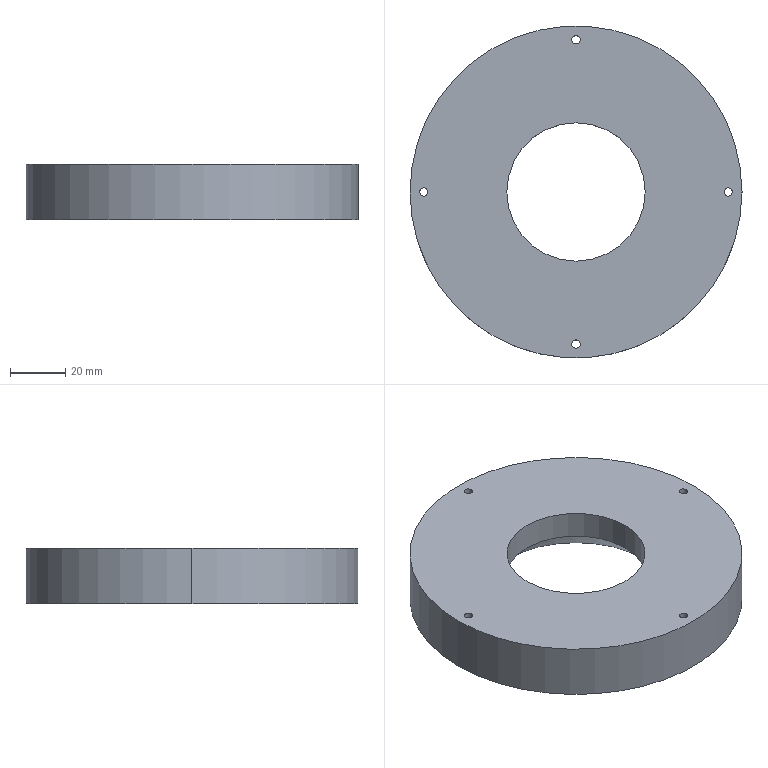Part | SolidWorks | features Chamfer 1, Extrusion 1, ICE 1 | 1 solid | 16 faces | box 120 x 120 x 20 mm | volume 177458 mm3 | cylinder 12 | cone 2 | plane 2 | commonest cylinder face diameters 3 x8 50 x2 120 x2
STEP:
#1=CARTESIAN_POINT('',(-1.5,55.,0.));
#2=VERTEX_POINT('',#1);
#3=CARTESIAN_POINT('',(1.5,55.,0.));
#4=VERTEX_POINT('',#3);
#5=CARTESIAN_POINT('',(0.,55.,0.));
#6=DIRECTION('',(0.,0.,1.));
#7=DIRECTION('',(1.,0.,0.));
#8=AXIS2_PLACEMENT_3D('',#5,#6,#7);
#9=CIRCLE('',#8,1.5);
#10=EDGE_CURVE('',#2,#4,#9,.T.);
#11=ORIENTED_EDGE('',*,*,#10,.F.);
#12=CARTESIAN_POINT('',(-1.5,55.,20.));
#13=VERTEX_POINT('',#12);
#14=CARTESIAN_POINT('',(-1.5,55.,-7.));
#15=DIRECTION('',(0.,0.,1.));
#16=VECTOR('',#15,1000.);
#17=LINE('',#14,#16);
#18=EDGE_CURVE('',#2,#13,#17,.T.);
#19=ORIENTED_EDGE('',*,*,#18,.T.);
#20=CARTESIAN_POINT('',(1.5,55.,20.));
#21=VERTEX_POINT('',#20);
#22=CARTESIAN_POINT('',(0.,55.,20.));
#23=DIRECTION('',(0.,0.,1.));
#24=DIRECTION('',(1.,0.,0.));
#25=AXIS2_PLACEMENT_3D('',#22,#23,#24);
#26=CIRCLE('',#25,1.5);
#27=EDGE_CURVE('',#13,#21,#26,.T.);
#28=ORIENTED_EDGE('',*,*,#27,.T.);
#29=CARTESIAN_POINT('',(1.5,55.,-7.));
#30=DIRECTION('',(0.,0.,1.));
#31=VECTOR('',#30,1000.);
#32=LINE('',#29,#31);
#33=EDGE_CURVE('',#4,#21,#32,.T.);
#34=ORIENTED_EDGE('',*,*,#33,.F.);
#35=EDGE_LOOP('',(#11,#19,#28,#34));
#36=FACE_OUTER_BOUND('',#35,.T.);
#37=CARTESIAN_POINT('',(0.,55.,-7.));
#38=DIRECTION('',(0.,0.,1.));
#39=DIRECTION('',(1.,0.,0.));
#40=AXIS2_PLACEMENT_3D('',#37,#38,#39);
#41=CYLINDRICAL_SURFACE('',#40,1.5);
#42=ADVANCED_FACE('',(#36),#41,.F.);
#43=CARTESIAN_POINT('',(53.5,0.,0.));
#44=VERTEX_POINT('',#43);
#45=CARTESIAN_POINT('',(56.5,0.,0.));
#46=VERTEX_POINT('',#45);
#47=CARTESIAN_POINT('',(55.,0.,0.));
#48=DIRECTION('',(0.,0.,1.));
#49=DIRECTION('',(1.,0.,0.));
#50=AXIS2_PLACEMENT_3D('',#47,#48,#49);
#51=CIRCLE('',#50,1.5);
#52=EDGE_CURVE('',#44,#46,#51,.T.);
#53=ORIENTED_EDGE('',*,*,#52,.F.);
#54=CARTESIAN_POINT('',(53.5,0.,20.));
#55=VERTEX_POINT('',#54);
#56=CARTESIAN_POINT('',(53.5,0.,-7.));
#57=DIRECTION('',(0.,0.,1.));
#58=VECTOR('',#57,1000.);
#59=LINE('',#56,#58);
#60=EDGE_CURVE('',#44,#55,#59,.T.);
#61=ORIENTED_EDGE('',*,*,#60,.T.);
#62=CARTESIAN_POINT('',(56.5,0.,20.));
#63=VERTEX_POINT('',#62);
#64=CARTESIAN_POINT('',(55.,0.,20.));
#65=DIRECTION('',(0.,0.,1.));
#66=DIRECTION('',(1.,0.,0.));
#67=AXIS2_PLACEMENT_3D('',#64,#65,#66);
#68=CIRCLE('',#67,1.5);
#69=EDGE_CURVE('',#55,#63,#68,.T.);
#70=ORIENTED_EDGE('',*,*,#69,.T.);
#71=CARTESIAN_POINT('',(56.5,0.,-7.));
#72=DIRECTION('',(0.,0.,1.));
#73=VECTOR('',#72,1000.);
#74=LINE('',#71,#73);
#75=EDGE_CURVE('',#46,#63,#74,.T.);
#76=ORIENTED_EDGE('',*,*,#75,.F.);
#77=EDGE_LOOP('',(#53,#61,#70,#76));
#78=FACE_OUTER_BOUND('',#77,.T.);
#79=CARTESIAN_POINT('',(55.,0.,-7.));
#80=DIRECTION('',(0.,0.,1.));
#81=DIRECTION('',(1.,0.,0.));
#82=AXIS2_PLACEMENT_3D('',#79,#80,#81);
#83=CYLINDRICAL_SURFACE('',#82,1.5);
#84=ADVANCED_FACE('',(#78),#83,.F.);
#85=CARTESIAN_POINT('',(-1.5,-55.,0.));
#86=VERTEX_POINT('',#85);
#87=CARTESIAN_POINT('',(1.5,-55.,0.));
#88=VERTEX_POINT('',#87);
#89=CARTESIAN_POINT('',(0.,-55.,0.));
#90=DIRECTION('',(0.,0.,1.));
#91=DIRECTION('',(1.,0.,0.));
#92=AXIS2_PLACEMENT_3D('',#89,#90,#91);
#93=CIRCLE('',#92,1.5);
#94=EDGE_CURVE('',#86,#88,#93,.T.);
#95=ORIENTED_EDGE('',*,*,#94,.F.);
#96=CARTESIAN_POINT('',(-1.5,-55.,20.));
#97=VERTEX_POINT('',#96);
#98=CARTESIAN_POINT('',(-1.5,-55.,-7.));
#99=DIRECTION('',(0.,0.,1.));
#100=VECTOR('',#99,1000.);
#101=LINE('',#98,#100);
#102=EDGE_CURVE('',#86,#97,#101,.T.);
#103=ORIENTED_EDGE('',*,*,#102,.T.);
#104=CARTESIAN_POINT('',(1.5,-55.,20.));
#105=VERTEX_POINT('',#104);
#106=CARTESIAN_POINT('',(0.,-55.,20.));
#107=DIRECTION('',(0.,0.,1.));
#108=DIRECTION('',(1.,0.,0.));
#109=AXIS2_PLACEMENT_3D('',#106,#107,#108);
#110=CIRCLE('',#109,1.5);
#111=EDGE_CURVE('',#97,#105,#110,.T.);
#112=ORIENTED_EDGE('',*,*,#111,.T.);
#113=CARTESIAN_POINT('',(1.5,-55.,-7.));
#114=DIRECTION('',(0.,0.,1.));
#115=VECTOR('',#114,1000.);
#116=LINE('',#113,#115);
#117=EDGE_CURVE('',#88,#105,#116,.T.);
#118=ORIENTED_EDGE('',*,*,#117,.F.);
#119=EDGE_LOOP('',(#95,#103,#112,#118));
#120=FACE_OUTER_BOUND('',#119,.T.);
#121=CARTESIAN_POINT('',(0.,-55.,-7.));
#122=DIRECTION('',(0.,0.,1.));
#123=DIRECTION('',(1.,0.,0.));
#124=AXIS2_PLACEMENT_3D('',#121,#122,#123);
#125=CYLINDRICAL_SURFACE('',#124,1.5);
#126=ADVANCED_FACE('',(#120),#125,.F.);
#127=CARTESIAN_POINT('',(-56.5,0.,0.));
#128=VERTEX_POINT('',#127);
#129=CARTESIAN_POINT('',(-53.5,0.,0.));
#130=VERTEX_POINT('',#129);
#131=CARTESIAN_POINT('',(-55.,0.,0.));
#132=DIRECTION('',(0.,0.,1.));
#133=DIRECTION('',(1.,0.,0.));
#134=AXIS2_PLACEMENT_3D('',#131,#132,#133);
#135=CIRCLE('',#134,1.5);
#136=EDGE_CURVE('',#128,#130,#135,.T.);
#137=ORIENTED_EDGE('',*,*,#136,.F.);
#138=CARTESIAN_POINT('',(-56.5,0.,20.));
#139=VERTEX_POINT('',#138);
#140=CARTESIAN_POINT('',(-56.5,0.,-7.));
#141=DIRECTION('',(0.,0.,1.));
#142=VECTOR('',#141,1000.);
#143=LINE('',#140,#142);
#144=EDGE_CURVE('',#128,#139,#143,.T.);
#145=ORIENTED_EDGE('',*,*,#144,.T.);
#146=CARTESIAN_POINT('',(-53.5,0.,20.));
#147=VERTEX_POINT('',#146);
#148=CARTESIAN_POINT('',(-55.,0.,20.));
#149=DIRECTION('',(0.,0.,1.));
#150=DIRECTION('',(1.,0.,0.));
#151=AXIS2_PLACEMENT_3D('',#148,#149,#150);
#152=CIRCLE('',#151,1.5);
#153=EDGE_CURVE('',#139,#147,#152,.T.);
#154=ORIENTED_EDGE('',*,*,#153,.T.);
#155=CARTESIAN_POINT('',(-53.5,0.,-7.));
#156=DIRECTION('',(0.,0.,1.));
#157=VECTOR('',#156,1000.);
#158=LINE('',#155,#157);
#159=EDGE_CURVE('',#130,#147,#158,.T.);
#160=ORIENTED_EDGE('',*,*,#159,.F.);
#161=EDGE_LOOP('',(#137,#145,#154,#160));
#162=FACE_OUTER_BOUND('',#161,.T.);
#163=CARTESIAN_POINT('',(-55.,0.,-7.));
#164=DIRECTION('',(0.,0.,1.));
#165=DIRECTION('',(1.,0.,0.));
#166=AXIS2_PLACEMENT_3D('',#163,#164,#165);
#167=CYLINDRICAL_SURFACE('',#166,1.5);
#168=ADVANCED_FACE('',(#162),#167,.F.);
#169=CARTESIAN_POINT('',(25.,0.,10.));
#170=VERTEX_POINT('',#169);
#171=CARTESIAN_POINT('',(-25.,0.,10.));
#172=VERTEX_POINT('',#171);
#173=CARTESIAN_POINT('',(0.,0.,10.));
#174=DIRECTION('',(0.,0.,-1.));
#175=DIRECTION('',(1.,0.,0.));
#176=AXIS2_PLACEMENT_3D('',#173,#174,#175);
#177=CIRCLE('',#176,25.);
#178=EDGE_CURVE('',#170,#172,#177,.T.);
#179=ORIENTED_EDGE('',*,*,#178,.F.);
#180=CARTESIAN_POINT('',(35.,0.,0.));
#181=VERTEX_POINT('',#180);
#182=CARTESIAN_POINT('',(35.,0.,0.));
#183=DIRECTION('',(0.7071,0.,-0.7071));
#184=VECTOR('',#183,1000.);
#185=LINE('',#182,#184);
#186=EDGE_CURVE('',#170,#181,#185,.T.);
#187=ORIENTED_EDGE('',*,*,#186,.T.);
#188=CARTESIAN_POINT('',(-35.,0.,0.));
#189=VERTEX_POINT('',#188);
#190=CARTESIAN_POINT('',(0.,0.,0.));
#191=DIRECTION('',(0.,0.,1.));
#192=DIRECTION('',(1.,0.,0.));
#193=AXIS2_PLACEMENT_3D('',#190,#191,#192);
#194=CIRCLE('',#193,35.);
#195=EDGE_CURVE('',#189,#181,#194,.T.);
#196=ORIENTED_EDGE('',*,*,#195,.F.);
#197=CARTESIAN_POINT('',(-35.,0.,0.));
#198=DIRECTION('',(-0.7071,0.,-0.7071));
#199=VECTOR('',#198,1000.);
#200=LINE('',#197,#199);
#201=EDGE_CURVE('',#172,#189,#200,.T.);
#202=ORIENTED_EDGE('',*,*,#201,.F.);
#203=EDGE_LOOP('',(#179,#187,#196,#202));
#204=FACE_OUTER_BOUND('',#203,.T.);
#205=CARTESIAN_POINT('',(0.,0.,0.));
#206=DIRECTION('',(0.,0.,-1.));
#207=DIRECTION('',(-1.,0.,0.));
#208=AXIS2_PLACEMENT_3D('',#205,#206,#207);
#209=CONICAL_SURFACE('',#208,35.,0.7854);
#210=ADVANCED_FACE('',(#204),#209,.F.);
#211=CARTESIAN_POINT('',(-25.,0.,20.));
#212=VERTEX_POINT('',#211);
#213=CARTESIAN_POINT('',(25.,0.,20.));
#214=VERTEX_POINT('',#213);
#215=CARTESIAN_POINT('',(0.,0.,20.));
#216=DIRECTION('',(0.,0.,1.));
#217=DIRECTION('',(1.,0.,0.));
#218=AXIS2_PLACEMENT_3D('',#215,#216,#217);
#219=CIRCLE('',#218,25.);
#220=EDGE_CURVE('',#212,#214,#219,.T.);
#221=ORIENTED_EDGE('',*,*,#220,.T.);
#222=CARTESIAN_POINT('',(25.,0.,20.));
#223=DIRECTION('',(0.,0.,-1.));
#224=VECTOR('',#223,1000.);
#225=LINE('',#222,#224);
#226=EDGE_CURVE('',#214,#170,#225,.T.);
#227=ORIENTED_EDGE('',*,*,#226,.T.);
#228=ORIENTED_EDGE('',*,*,#178,.T.);
#229=CARTESIAN_POINT('',(-25.,0.,20.));
#230=DIRECTION('',(0.,0.,-1.));
#231=VECTOR('',#230,1000.);
#232=LINE('',#229,#231);
#233=EDGE_CURVE('',#212,#172,#232,.T.);
#234=ORIENTED_EDGE('',*,*,#233,.F.);
#235=EDGE_LOOP('',(#221,#227,#228,#234));
#236=FACE_OUTER_BOUND('',#235,.T.);
#237=CARTESIAN_POINT('',(0.,0.,20.));
#238=DIRECTION('',(0.,0.,-1.));
#239=DIRECTION('',(-1.,0.,0.));
#240=AXIS2_PLACEMENT_3D('',#237,#238,#239);
#241=CYLINDRICAL_SURFACE('',#240,25.);
#242=ADVANCED_FACE('',(#236),#241,.F.);
#243=CARTESIAN_POINT('',(60.,0.,20.));
#244=VERTEX_POINT('',#243);
#245=CARTESIAN_POINT('',(-60.,0.,20.));
#246=VERTEX_POINT('',#245);
#247=CARTESIAN_POINT('',(0.,0.,20.));
#248=DIRECTION('',(0.,0.,1.));
#249=DIRECTION('',(1.,0.,0.));
#250=AXIS2_PLACEMENT_3D('',#247,#248,#249);
#251=CIRCLE('',#250,60.);
#252=EDGE_CURVE('',#244,#246,#251,.T.);
#253=ORIENTED_EDGE('',*,*,#252,.F.);
#254=CARTESIAN_POINT('',(60.,0.,0.));
#255=VERTEX_POINT('',#254);
#256=CARTESIAN_POINT('',(60.,0.,20.));
#257=DIRECTION('',(0.,0.,-1.));
#258=VECTOR('',#257,1000.);
#259=LINE('',#256,#258);
#260=EDGE_CURVE('',#244,#255,#259,.T.);
#261=ORIENTED_EDGE('',*,*,#260,.T.);
#262=CARTESIAN_POINT('',(-60.,0.,0.));
#263=VERTEX_POINT('',#262);
#264=CARTESIAN_POINT('',(0.,0.,0.));
#265=DIRECTION('',(0.,0.,1.));
#266=DIRECTION('',(1.,0.,0.));
#267=AXIS2_PLACEMENT_3D('',#264,#265,#266);
#268=CIRCLE('',#267,60.);
#269=EDGE_CURVE('',#255,#263,#268,.T.);
#270=ORIENTED_EDGE('',*,*,#269,.T.);
#271=CARTESIAN_POINT('',(-60.,0.,20.));
#272=DIRECTION('',(0.,0.,-1.));
#273=VECTOR('',#272,1000.);
#274=LINE('',#271,#273);
#275=EDGE_CURVE('',#246,#263,#274,.T.);
#276=ORIENTED_EDGE('',*,*,#275,.F.);
#277=EDGE_LOOP('',(#253,#261,#270,#276));
#278=FACE_OUTER_BOUND('',#277,.T.);
#279=CARTESIAN_POINT('',(0.,0.,20.));
#280=DIRECTION('',(0.,0.,-1.));
#281=DIRECTION('',(-1.,0.,0.));
#282=AXIS2_PLACEMENT_3D('',#279,#280,#281);
#283=CYLINDRICAL_SURFACE('',#282,60.);
#284=ADVANCED_FACE('',(#278),#283,.T.);
#285=CARTESIAN_POINT('',(0.,55.,20.));
#286=DIRECTION('',(0.,0.,1.));
#287=DIRECTION('',(1.,0.,0.));
#288=AXIS2_PLACEMENT_3D('',#285,#286,#287);
#289=CIRCLE('',#288,1.5);
#290=EDGE_CURVE('',#21,#13,#289,.T.);
#291=ORIENTED_EDGE('',*,*,#290,.F.);
#292=ORIENTED_EDGE('',*,*,#27,.F.);
#293=EDGE_LOOP('',(#291,#292));
#294=FACE_BOUND('',#293,.T.);
#295=CARTESIAN_POINT('',(55.,0.,20.));
#296=DIRECTION('',(0.,0.,1.));
#297=DIRECTION('',(1.,0.,0.));
#298=AXIS2_PLACEMENT_3D('',#295,#296,#297);
#299=CIRCLE('',#298,1.5);
#300=EDGE_CURVE('',#63,#55,#299,.T.);
#301=ORIENTED_EDGE('',*,*,#300,.F.);
#302=ORIENTED_EDGE('',*,*,#69,.F.);
#303=EDGE_LOOP('',(#301,#302));
#304=FACE_BOUND('',#303,.T.);
#305=CARTESIAN_POINT('',(0.,-55.,20.));
#306=DIRECTION('',(0.,0.,1.));
#307=DIRECTION('',(1.,0.,0.));
#308=AXIS2_PLACEMENT_3D('',#305,#306,#307);
#309=CIRCLE('',#308,1.5);
#310=EDGE_CURVE('',#105,#97,#309,.T.);
#311=ORIENTED_EDGE('',*,*,#310,.F.);
#312=ORIENTED_EDGE('',*,*,#111,.F.);
#313=EDGE_LOOP('',(#311,#312));
#314=FACE_BOUND('',#313,.T.);
#315=CARTESIAN_POINT('',(-55.,0.,20.));
#316=DIRECTION('',(0.,0.,1.));
#317=DIRECTION('',(1.,0.,0.));
#318=AXIS2_PLACEMENT_3D('',#315,#316,#317);
#319=CIRCLE('',#318,1.5);
#320=EDGE_CURVE('',#147,#139,#319,.T.);
#321=ORIENTED_EDGE('',*,*,#320,.F.);
#322=ORIENTED_EDGE('',*,*,#153,.F.);
#323=EDGE_LOOP('',(#321,#322));
#324=FACE_BOUND('',#323,.T.);
#325=CARTESIAN_POINT('',(0.,0.,20.));
#326=DIRECTION('',(0.,0.,1.));
#327=DIRECTION('',(1.,0.,0.));
#328=AXIS2_PLACEMENT_3D('',#325,#326,#327);
#329=CIRCLE('',#328,60.);
#330=EDGE_CURVE('',#246,#244,#329,.T.);
#331=ORIENTED_EDGE('',*,*,#330,.T.);
#332=ORIENTED_EDGE('',*,*,#252,.T.);
#333=EDGE_LOOP('',(#331,#332));
#334=FACE_OUTER_BOUND('',#333,.T.);
#335=ORIENTED_EDGE('',*,*,#220,.F.);
#336=CARTESIAN_POINT('',(0.,0.,20.));
#337=DIRECTION('',(0.,0.,1.));
#338=DIRECTION('',(1.,0.,0.));
#339=AXIS2_PLACEMENT_3D('',#336,#337,#338);
#340=CIRCLE('',#339,25.);
#341=EDGE_CURVE('',#214,#212,#340,.T.);
#342=ORIENTED_EDGE('',*,*,#341,.F.);
#343=EDGE_LOOP('',(#335,#342));
#344=FACE_BOUND('',#343,.T.);
#345=CARTESIAN_POINT('',(0.,0.,20.));
#346=DIRECTION('',(0.,0.,1.));
#347=DIRECTION('',(1.,0.,0.));
#348=AXIS2_PLACEMENT_3D('',#345,#346,#347);
#349=PLANE('',#348);
#350=ADVANCED_FACE('',(#294,#304,#314,#324,#334,#344),#349,.T.);
#351=CARTESIAN_POINT('',(0.,55.,0.));
#352=DIRECTION('',(0.,0.,1.));
#353=DIRECTION('',(1.,0.,0.));
#354=AXIS2_PLACEMENT_3D('',#351,#352,#353);
#355=CIRCLE('',#354,1.5);
#356=EDGE_CURVE('',#4,#2,#355,.T.);
#357=ORIENTED_EDGE('',*,*,#356,.T.);
#358=ORIENTED_EDGE('',*,*,#10,.T.);
#359=EDGE_LOOP('',(#357,#358));
#360=FACE_BOUND('',#359,.T.);
#361=CARTESIAN_POINT('',(55.,0.,0.));
#362=DIRECTION('',(0.,0.,1.));
#363=DIRECTION('',(1.,0.,0.));
#364=AXIS2_PLACEMENT_3D('',#361,#362,#363);
#365=CIRCLE('',#364,1.5);
#366=EDGE_CURVE('',#46,#44,#365,.T.);
#367=ORIENTED_EDGE('',*,*,#366,.T.);
#368=ORIENTED_EDGE('',*,*,#52,.T.);
#369=EDGE_LOOP('',(#367,#368));
#370=FACE_BOUND('',#369,.T.);
#371=CARTESIAN_POINT('',(0.,-55.,0.));
#372=DIRECTION('',(0.,0.,1.));
#373=DIRECTION('',(1.,0.,0.));
#374=AXIS2_PLACEMENT_3D('',#371,#372,#373);
#375=CIRCLE('',#374,1.5);
#376=EDGE_CURVE('',#88,#86,#375,.T.);
#377=ORIENTED_EDGE('',*,*,#376,.T.);
#378=ORIENTED_EDGE('',*,*,#94,.T.);
#379=EDGE_LOOP('',(#377,#378));
#380=FACE_BOUND('',#379,.T.);
#381=CARTESIAN_POINT('',(-55.,0.,0.));
#382=DIRECTION('',(0.,0.,1.));
#383=DIRECTION('',(1.,0.,0.));
#384=AXIS2_PLACEMENT_3D('',#381,#382,#383);
#385=CIRCLE('',#384,1.5);
#386=EDGE_CURVE('',#130,#128,#385,.T.);
#387=ORIENTED_EDGE('',*,*,#386,.T.);
#388=ORIENTED_EDGE('',*,*,#136,.T.);
#389=EDGE_LOOP('',(#387,#388));
#390=FACE_BOUND('',#389,.T.);
#391=ORIENTED_EDGE('',*,*,#195,.T.);
#392=CARTESIAN_POINT('',(0.,0.,0.));
#393=DIRECTION('',(0.,0.,1.));
#394=DIRECTION('',(1.,0.,0.));
#395=AXIS2_PLACEMENT_3D('',#392,#393,#394);
#396=CIRCLE('',#395,35.);
#397=EDGE_CURVE('',#181,#189,#396,.T.);
#398=ORIENTED_EDGE('',*,*,#397,.T.);
#399=EDGE_LOOP('',(#391,#398));
#400=FACE_BOUND('',#399,.T.);
#401=CARTESIAN_POINT('',(0.,0.,0.));
#402=DIRECTION('',(0.,0.,1.));
#403=DIRECTION('',(1.,0.,0.));
#404=AXIS2_PLACEMENT_3D('',#401,#402,#403);
#405=CIRCLE('',#404,60.);
#406=EDGE_CURVE('',#263,#255,#405,.T.);
#407=ORIENTED_EDGE('',*,*,#406,.F.);
#408=ORIENTED_EDGE('',*,*,#269,.F.);
#409=EDGE_LOOP('',(#407,#408));
#410=FACE_OUTER_BOUND('',#409,.T.);
#411=CARTESIAN_POINT('',(0.,0.,0.));
#412=DIRECTION('',(0.,0.,1.));
#413=DIRECTION('',(1.,0.,0.));
#414=AXIS2_PLACEMENT_3D('',#411,#412,#413);
#415=PLANE('',#414);
#416=ADVANCED_FACE('',(#360,#370,#380,#390,#400,#410),#415,.F.);
#417=ORIENTED_EDGE('',*,*,#260,.F.);
#418=ORIENTED_EDGE('',*,*,#330,.F.);
#419=ORIENTED_EDGE('',*,*,#275,.T.);
#420=ORIENTED_EDGE('',*,*,#406,.T.);
#421=EDGE_LOOP('',(#417,#418,#419,#420));
#422=FACE_OUTER_BOUND('',#421,.T.);
#423=CARTESIAN_POINT('',(0.,0.,20.));
#424=DIRECTION('',(0.,0.,-1.));
#425=DIRECTION('',(-1.,0.,0.));
#426=AXIS2_PLACEMENT_3D('',#423,#424,#425);
#427=CYLINDRICAL_SURFACE('',#426,60.);
#428=ADVANCED_FACE('',(#422),#427,.T.);
#429=ORIENTED_EDGE('',*,*,#226,.F.);
#430=ORIENTED_EDGE('',*,*,#341,.T.);
#431=ORIENTED_EDGE('',*,*,#233,.T.);
#432=CARTESIAN_POINT('',(0.,0.,10.));
#433=DIRECTION('',(0.,0.,-1.));
#434=DIRECTION('',(1.,0.,0.));
#435=AXIS2_PLACEMENT_3D('',#432,#433,#434);
#436=CIRCLE('',#435,25.);
#437=EDGE_CURVE('',#172,#170,#436,.T.);
#438=ORIENTED_EDGE('',*,*,#437,.T.);
#439=EDGE_LOOP('',(#429,#430,#431,#438));
#440=FACE_OUTER_BOUND('',#439,.T.);
#441=CARTESIAN_POINT('',(0.,0.,20.));
#442=DIRECTION('',(0.,0.,-1.));
#443=DIRECTION('',(-1.,0.,0.));
#444=AXIS2_PLACEMENT_3D('',#441,#442,#443);
#445=CYLINDRICAL_SURFACE('',#444,25.);
#446=ADVANCED_FACE('',(#440),#445,.F.);
#447=ORIENTED_EDGE('',*,*,#186,.F.);
#448=ORIENTED_EDGE('',*,*,#437,.F.);
#449=ORIENTED_EDGE('',*,*,#201,.T.);
#450=ORIENTED_EDGE('',*,*,#397,.F.);
#451=EDGE_LOOP('',(#447,#448,#449,#450));
#452=FACE_OUTER_BOUND('',#451,.T.);
#453=CARTESIAN_POINT('',(0.,0.,0.));
#454=DIRECTION('',(0.,0.,-1.));
#455=DIRECTION('',(-1.,0.,0.));
#456=AXIS2_PLACEMENT_3D('',#453,#454,#455);
#457=CONICAL_SURFACE('',#456,35.,0.7854);
#458=ADVANCED_FACE('',(#452),#457,.F.);
#459=ORIENTED_EDGE('',*,*,#144,.F.);
#460=ORIENTED_EDGE('',*,*,#386,.F.);
#461=ORIENTED_EDGE('',*,*,#159,.T.);
#462=ORIENTED_EDGE('',*,*,#320,.T.);
#463=EDGE_LOOP('',(#459,#460,#461,#462));
#464=FACE_OUTER_BOUND('',#463,.T.);
#465=CARTESIAN_POINT('',(-55.,0.,-7.));
#466=DIRECTION('',(0.,0.,1.));
#467=DIRECTION('',(1.,0.,0.));
#468=AXIS2_PLACEMENT_3D('',#465,#466,#467);
#469=CYLINDRICAL_SURFACE('',#468,1.5);
#470=ADVANCED_FACE('',(#464),#469,.F.);
#471=ORIENTED_EDGE('',*,*,#102,.F.);
#472=ORIENTED_EDGE('',*,*,#376,.F.);
#473=ORIENTED_EDGE('',*,*,#117,.T.);
#474=ORIENTED_EDGE('',*,*,#310,.T.);
#475=EDGE_LOOP('',(#471,#472,#473,#474));
#476=FACE_OUTER_BOUND('',#475,.T.);
#477=CARTESIAN_POINT('',(0.,-55.,-7.));
#478=DIRECTION('',(0.,0.,1.));
#479=DIRECTION('',(1.,0.,0.));
#480=AXIS2_PLACEMENT_3D('',#477,#478,#479);
#481=CYLINDRICAL_SURFACE('',#480,1.5);
#482=ADVANCED_FACE('',(#476),#481,.F.);
#483=ORIENTED_EDGE('',*,*,#60,.F.);
#484=ORIENTED_EDGE('',*,*,#366,.F.);
#485=ORIENTED_EDGE('',*,*,#75,.T.);
#486=ORIENTED_EDGE('',*,*,#300,.T.);
#487=EDGE_LOOP('',(#483,#484,#485,#486));
#488=FACE_OUTER_BOUND('',#487,.T.);
#489=CARTESIAN_POINT('',(55.,0.,-7.));
#490=DIRECTION('',(0.,0.,1.));
#491=DIRECTION('',(1.,0.,0.));
#492=AXIS2_PLACEMENT_3D('',#489,#490,#491);
#493=CYLINDRICAL_SURFACE('',#492,1.5);
#494=ADVANCED_FACE('',(#488),#493,.F.);
#495=ORIENTED_EDGE('',*,*,#18,.F.);
#496=ORIENTED_EDGE('',*,*,#356,.F.);
#497=ORIENTED_EDGE('',*,*,#33,.T.);
#498=ORIENTED_EDGE('',*,*,#290,.T.);
#499=EDGE_LOOP('',(#495,#496,#497,#498));
#500=FACE_OUTER_BOUND('',#499,.T.);
#501=CARTESIAN_POINT('',(0.,55.,-7.));
#502=DIRECTION('',(0.,0.,1.));
#503=DIRECTION('',(1.,0.,0.));
#504=AXIS2_PLACEMENT_3D('',#501,#502,#503);
#505=CYLINDRICAL_SURFACE('',#504,1.5);
#506=ADVANCED_FACE('',(#500),#505,.F.);
#507=CLOSED_SHELL('',(#42,#84,#126,#168,#210,#242,#284,#350,#416,#428,#446,#458,#470,#482,#494,#506));
#508=MANIFOLD_SOLID_BREP('',#507);
#509=CARTESIAN_POINT('',(0.,0.,0.));
#510=DIRECTION('',(0.,0.,1.));
#511=DIRECTION('',(1.,0.,0.));
#512=AXIS2_PLACEMENT_3D('',#509,#510,#511);
#513=(LENGTH_UNIT()NAMED_UNIT(*)SI_UNIT(.MILLI.,.METRE.));
#514=UNCERTAINTY_MEASURE_WITH_UNIT(LENGTH_MEASURE(0.00001),#513,'','');
#515=(NAMED_UNIT(*)PLANE_ANGLE_UNIT()SI_UNIT($,.RADIAN.));
#516=(NAMED_UNIT(*)SI_UNIT($,.STERADIAN.)SOLID_ANGLE_UNIT());
#517=(GEOMETRIC_REPRESENTATION_CONTEXT(3)GLOBAL_UNCERTAINTY_ASSIGNED_CONTEXT((#514))GLOBAL_UNIT_ASSIGNED_CONTEXT((#513,#515,#516))REPRESENTATION_CONTEXT('',''));
#518=ADVANCED_BREP_SHAPE_REPRESENTATION('',(#508,#512),#517);